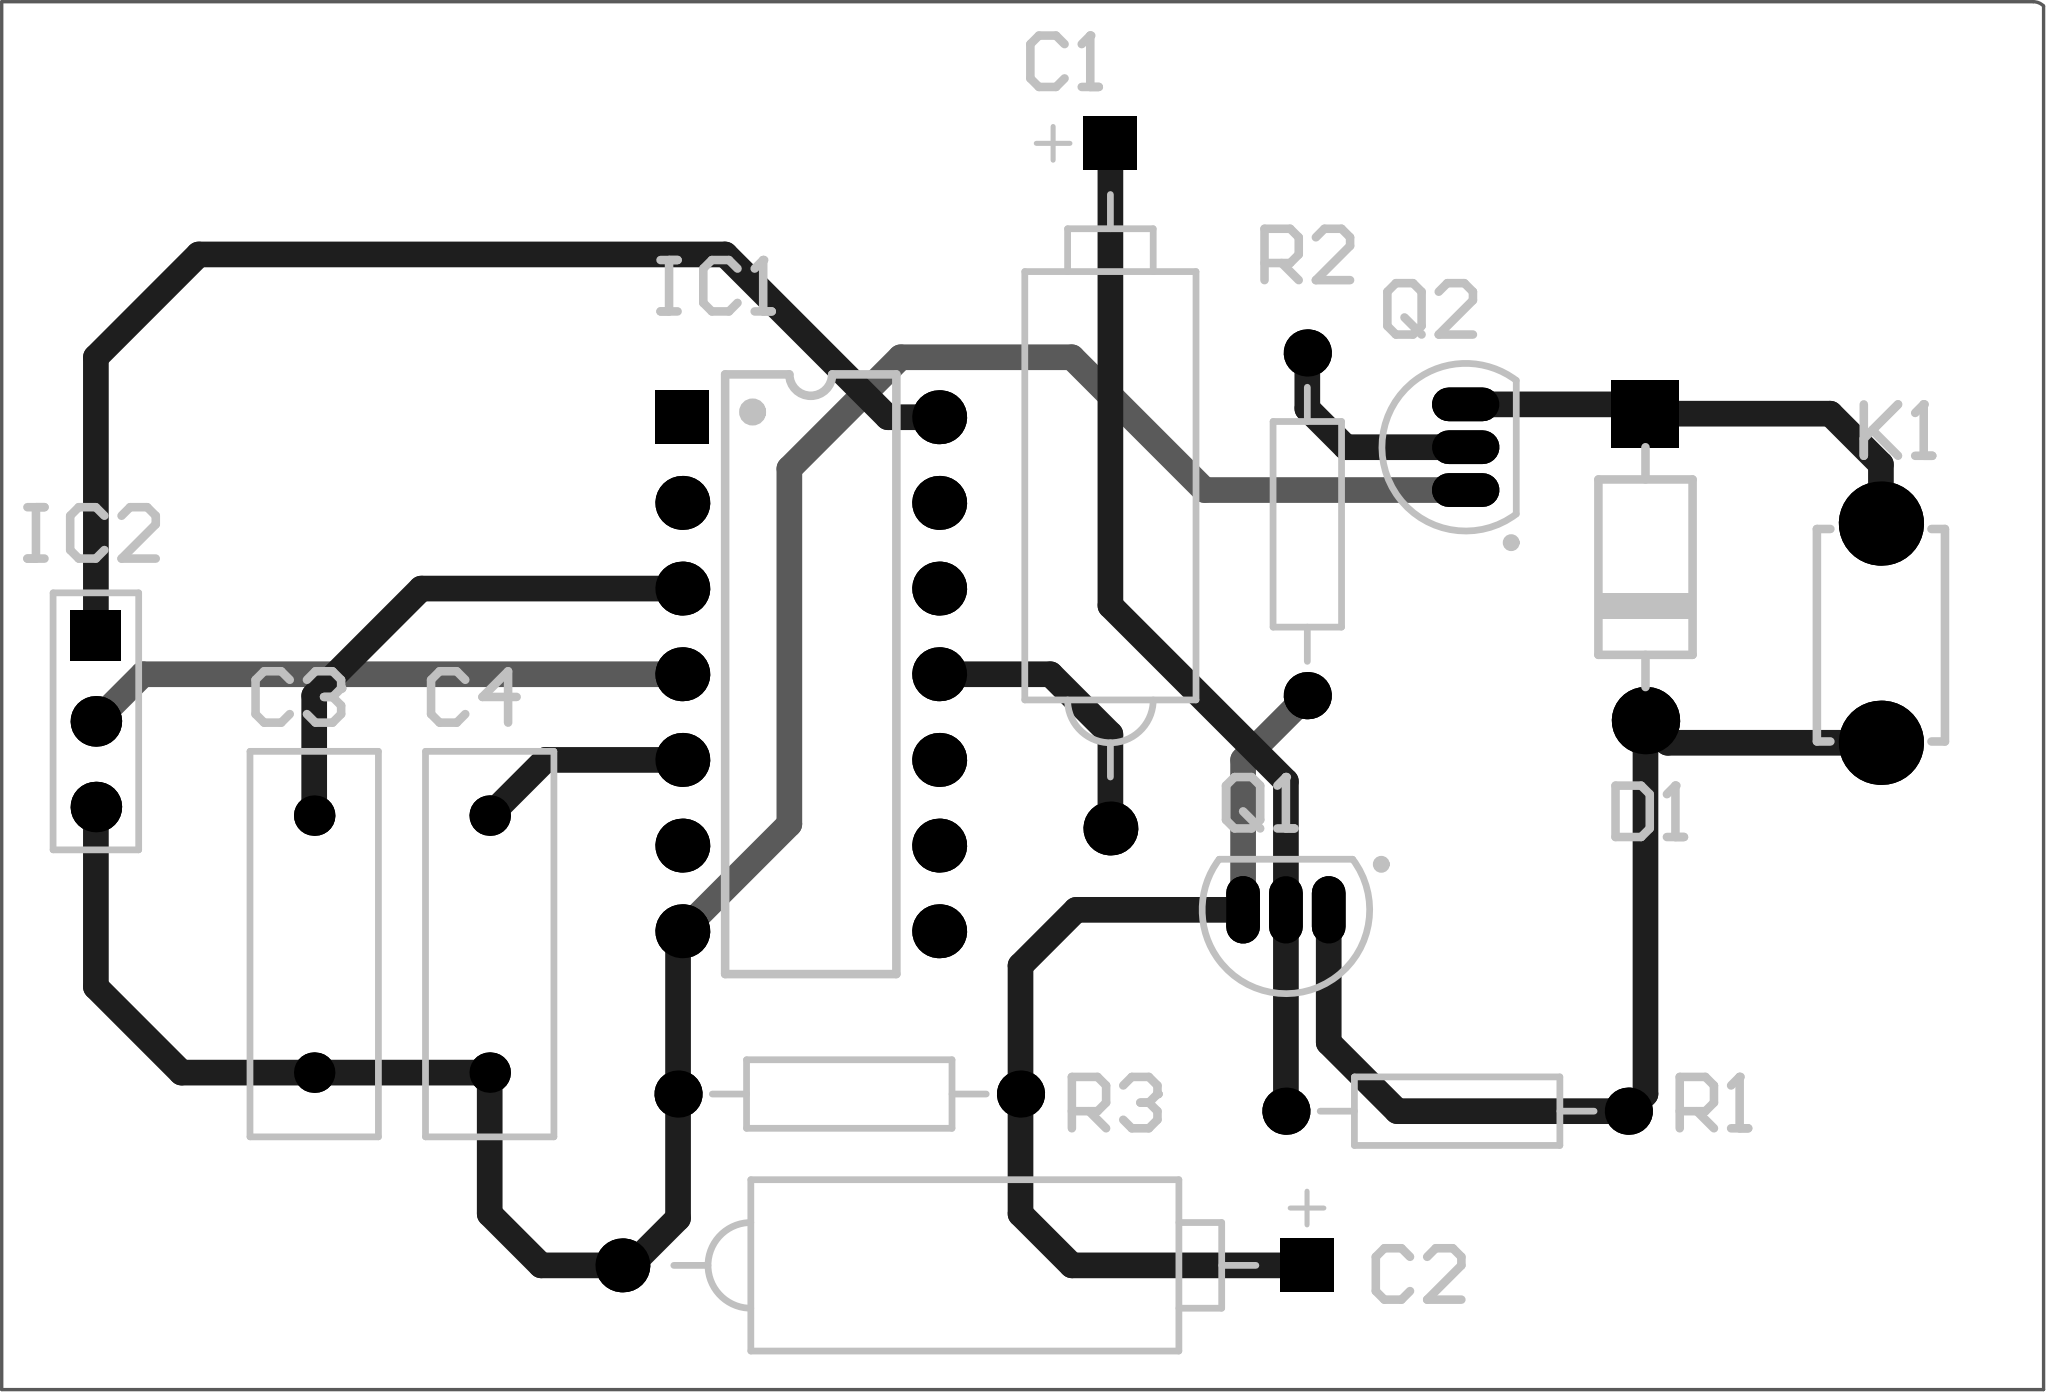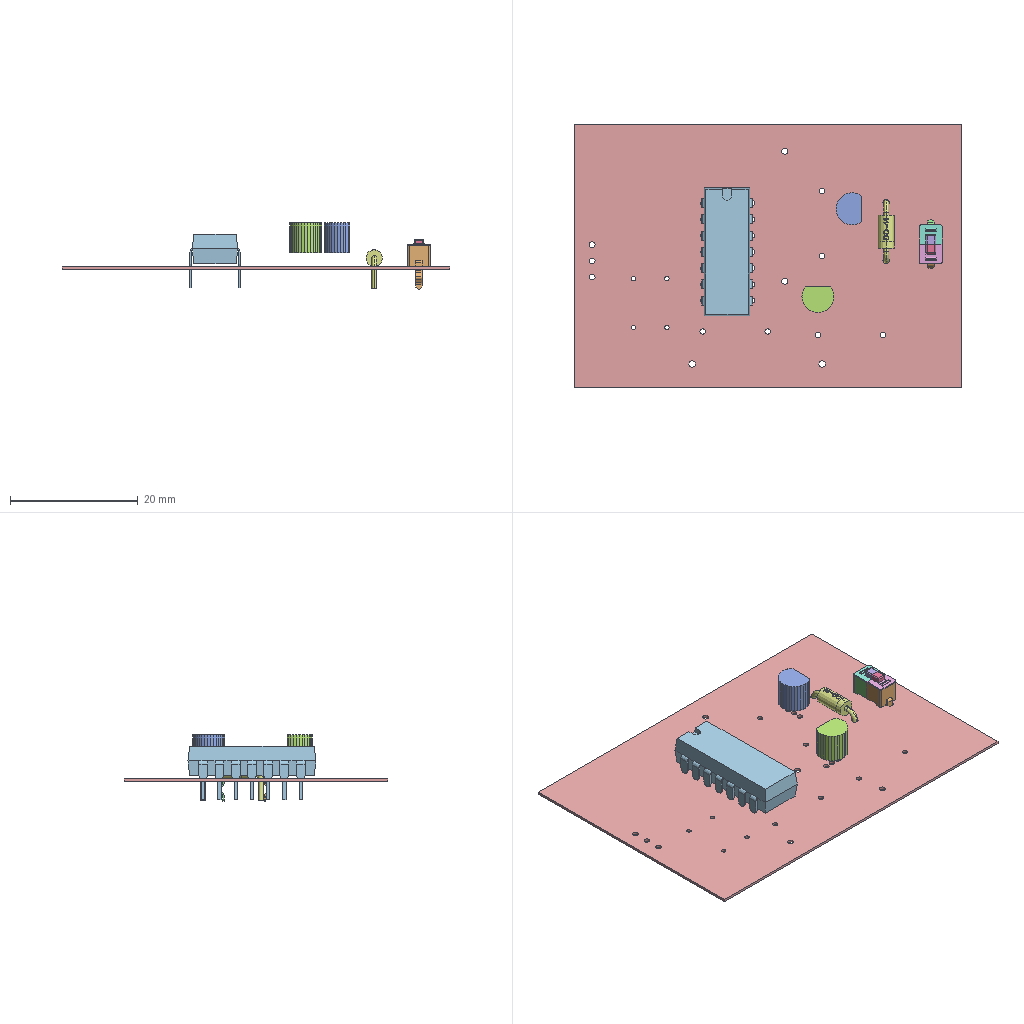Circuit board layout | Altium Designer | box 60.6 x 41.1 x 10.3 mm
Layer stack:
# Altium Designer layer stack of  (unit mm; dielectric type: 0 none, 1 core, 2 prepreg, 3 surface material)
index,name,kind,layer,copper_thickness_mm,dielectric_type,dielectric_thickness_mm,dielectric_material,dielectric_constant
0,Top Paste,other,,,,,,
1,Top Overlay,other,,,,,,
2,Top Solder,dielectric,,,3,0.0102,Solder Resist,3.5
3,Top Layer,copper,Top Layer,0.0356,,,,
4,Dielectric 1,dielectric,,,0,0.32,FR-4,4.8
5,Bottom Layer,copper,Bottom Layer,0.0356,,,,
6,Bottom Solder,dielectric,,,3,0.0102,Solder Resist,3.5
7,Bottom Overlay,other,,,,,,
8,Bottom Paste,other,,,,,,
# drill layer pairs: low layer,high layer
drill_pair,Top Layer,Bottom Layer
Part placement:
Designator,Comment,Layer,Footprint,Center-X(mm),Center-Y(mm),Rotation
R3,100K,TopLayer,AXIAL-0.4,121.285,33.782,360
R2,510,TopLayer,AXIAL-0.4,134.874,50.673,270
R1,10K,TopLayer,AXIAL-0.4,139.319,33.274,360
Q2,8050,TopLayer,TO-92A,139.573,52.959,0
Q1,9012,TopLayer,TO-92A,134.239,39.243,90
K1,KEY,TopLayer,DIP-3X6X4.3,151.892,47.446,270
IC2,BA5302,TopLayer,HDR1X3,98.933,44.831,270
IC1,LC9305,TopLayer,DIP14,120.142,46.228,0
D1,1N4001,TopLayer,DO-41,144.907,49.403,270
C4,3300PF,TopLayer,RAD-0.3,110.617,38.227,90
C3,0.022UF,TopLayer,RAD-0.3,105.41,38.227,90
C2,100UF,TopLayer,POLAR0.8,124.714,28.702,360
C1,1UF,TopLayer,POLAR0.8,129.032,51.816,90
Pad and via stacks:
# Altium Designer via and pad stacks of  (unit mm). Each distinct definition once, with the count of objects using it.
# via: kind,start_layer,end_layer,hole_mm,diameter_mm,mode(0 simple;1 top-mid-bottom;2 full stack),diameter_per_layer,count,example_net
# pad: kind,layer,hole_mm,hole_type(0 round;1 square;2 slot),plating,top_size,top_shape(1 round;2 rect;3 octagon;9 rounded rect),mid_size,bottom_size,mode,footprint,size_per_layer,count,example
pad,Multi-Layer,1,0,plated,1.6x1.6,1,1.6x1.6,1.6x1.6,0,POLAR0.8,,2,C2.2
pad,Multi-Layer,1,0,plated,1.6x1.6,2,1.6x1.6,1.6x1.6,0,POLAR0.8,,2,C2.1
pad,Multi-Layer,0.7,0,plated,1.2x1.2,1,1.2x1.2,1.2x1.2,0,RAD-0.3,,4,C4.2
pad,Multi-Layer,1,0,plated,2x2,1,2x2,2x2,0,DO-41,,1,D1.2
pad,Multi-Layer,1,0,plated,2x2,2,2x2,2x2,0,DO-41,,1,D1.1
pad,Multi-Layer,0.8128,0,plated,1.6x1.6,1,1.6x1.6,1.6x1.6,0,DIP14,,13,IC1.14
pad,Multi-Layer,0.8128,0,plated,1.6x1.6,2,1.6x1.6,1.6x1.6,0,DIP14,,1,IC1.1
pad,Multi-Layer,0.9,0,plated,1.5x1.5,2,1.5x1.5,1.5x1.5,0,HDR1X3,,1,IC2.1
pad,Multi-Layer,0.9,0,plated,1.5x1.5,1,1.5x1.5,1.5x1.5,0,HDR1X3,,2,IC2.2
pad,Multi-Layer,1.2,0,plated,2.5x2.5,1,2.5x2.5,2.5x2.5,0,DIP-3X6X4.3,,2,K1.1
pad,Multi-Layer,0.9,0,plated,2x1,1,2x1,2x1,0,TO-92A,,6,Q2.3
pad,Multi-Layer,0.85,0,plated,1.4x1.4,1,1.4x1.4,1.4x1.4,0,AXIAL-0.4,,6,R3.1
Design rules, without the lines most boards share:
# Altium Designer design rules of  (exported by Altium Designer, unit mm)
# columns: name | kind | enabled | priority | scope1 | scope2 | descriptor | typed fields (field=value)
SilkToSilkClearance | 55 | enabled | 1 | All | All | Silk to Silk (Clearance=0mil) (All),(All) |
SilkToSolderMaskClearance | 54 | enabled | 1 | IsPad | All | Silk To Solder Mask (Clearance=0mil) (IsPad),(All) |
MinimumSolderMaskSliver | 53 | enabled | 1 | All | All | Minimum Solder Mask Sliver (Gap=0mil) (All),(All) |
HoleToHoleClearance | 52 | enabled | 1 | All | All | Hole To Hole Clearance (Gap=10mil) (All),(All) | gap=0.254
DiffPairsRouting | 51 | enabled | 1 | All | All | Differential Pairs Uncoupled Length using the Gap Constraints (Min=10mil) (Max=10mil) (Prefered=10mil)  and Width Constraints (Min=15mil) (Max=15mil) (Prefered=15mil) (All) |
SolderMaskExpansion | 13 | enabled | 1 | All | All | Solder Mask Expansion (Expansion =4mil) (All) | expansion=0.1016
PasteMaskExpansion | 14 | enabled | 1 | All | All | Paste Mask Expansion (Expansion =0mil) (All) | expansion=0
RoutingVias | 11 | enabled | 1 | All | All | Routing Via (MinHoleWidth=28mil) (MaxHoleWidth=28mil) (PreferredHoleWidth=28mil) (MinWidth=50mil) (MaxWidth=50mil) (PreferedWidth=50mil) (All) | via_min_hole=0.7112 via_max_hole=0.7112 via_preferred_diameter=1.27 via_preferred_hole=0.7112
Width | 2 | enabled | 1 | All | All | Width Constraint (Min=10mil) (Max=30mil) (Preferred=10mil) (All) |
PolygonConnect | 20 | enabled | 1 | All | All | Polygon Connect Rule(Relief Connect )(Conductor Width=10mil) (Relief Angle=90 Angle) (Entries=4) (Air Gap Width=10mil) (All),(All) | connect_style(0=relief,1=direct,2=none)=0 relief_conductor_width=0.254 relief_entries=4
PlaneConnect | 6 | enabled | 1 | All | All | Power Plane Connect Rule(Relief Connect )(Expansion=20mil) (Conductor Width=10mil) (Air Gap=10mil) (Entries=4) (All) | relief_conductor_width=0.254 relief_entries=4 relief_expansion=0.508
Clearance | 0 | enabled | 1 | All | All | Clearance Constraint (Gap=10mil) (All),(All) | gap=0.254
Classes set for this board:
# Altium Designer classes of  (member kind: 0 net, 1 component, 2 from-to, 3 pad, 4 layer, 5 differential pair, 6 design channel, 7 polygon, 8 structure, 9 xSignal)
# columns: class name | member kind | superclass | members
Sheet1 | 1 | no | C1; C2; C3; C4; D1; IC1; IC2; K1; Q1; Q2; R1; R2; R3;